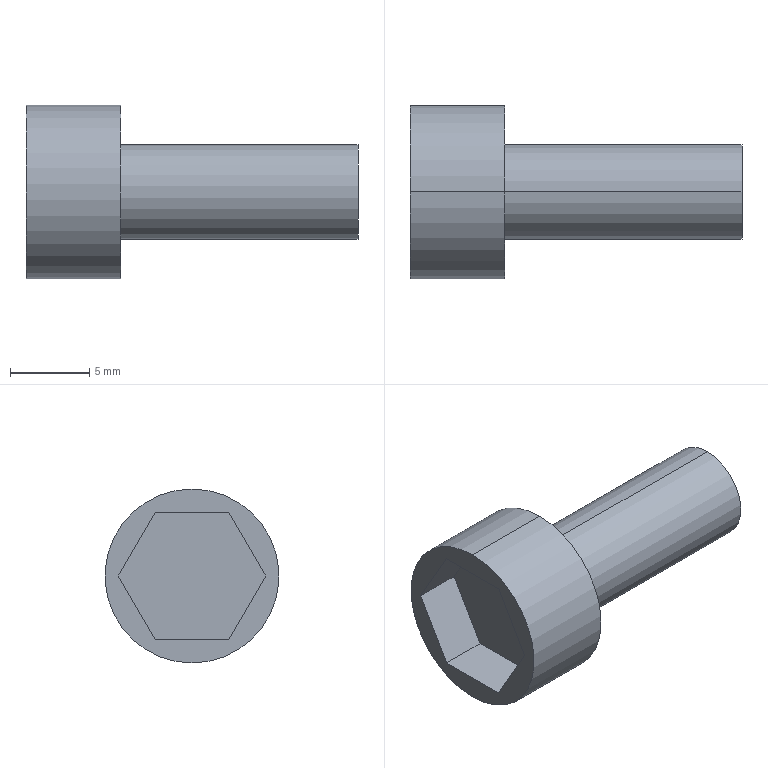Part | STEP file | M6 screw | 1 solid | 14 faces | box 21 x 11 x 11 mm | volume 825.269 mm3 | plane 10 | cylinder 4 | commonest cylinder face diameters 6 x2 11 x2
STEP:
#1=CARTESIAN_POINT('',(0.,0.,0.));
#2=DIRECTION('',(0.,0.,1.));
#3=DIRECTION('',(1.,0.,0.));
#4=AXIS2_PLACEMENT_3D('',#1,#2,#3);
#5=CARTESIAN_POINT('',(-7.171,-5.398,5.5));
#6=VERTEX_POINT('',#5);
#7=CARTESIAN_POINT('',(-7.171,-5.398,-5.5));
#8=VERTEX_POINT('',#7);
#9=CARTESIAN_POINT('',(-7.171,-5.398,0.));
#10=DIRECTION('',(-1.,0.,0.));
#11=DIRECTION('',(0.,0.,1.));
#12=AXIS2_PLACEMENT_3D('',#9,#10,#11);
#13=CIRCLE('',#12,5.5);
#14=CARTESIAN_POINT('',(-13.171,-5.398,0.));
#15=DIRECTION('',(-1.,0.,0.));
#16=DIRECTION('',(0.,0.,1.));
#17=AXIS2_PLACEMENT_3D('',#14,#15,#16);
#18=CYLINDRICAL_SURFACE('',#17,5.5);
#19=CARTESIAN_POINT('',(0.,-6.));
#20=DIRECTION('',(1.,0.));
#21=VECTOR('',#20,1.);
#22=LINE('',#19,#21);
#23=(GEOMETRIC_REPRESENTATION_CONTEXT(2)PARAMETRIC_REPRESENTATION_CONTEXT()REPRESENTATION_CONTEXT('',''));
#24=DEFINITIONAL_REPRESENTATION('',(#22),#23);
#25=PCURVE('',#18,#24);
#26=CARTESIAN_POINT('',(-7.171,0.102,0.));
#27=DIRECTION('',(-1.,0.,0.));
#28=DIRECTION('',(0.,0.,1.));
#29=AXIS2_PLACEMENT_3D('',#26,#27,#28);
#30=PLANE('',#29);
#31=CARTESIAN_POINT('',(0.,-5.5));
#32=DIRECTION('',(1.,0.));
#33=AXIS2_PLACEMENT_2D('',#31,#32);
#34=CIRCLE('',#33,5.5);
#35=(GEOMETRIC_REPRESENTATION_CONTEXT(2)PARAMETRIC_REPRESENTATION_CONTEXT()REPRESENTATION_CONTEXT('',''));
#36=DEFINITIONAL_REPRESENTATION('',(#34),#35);
#37=PCURVE('',#30,#36);
#38=SURFACE_CURVE('',#13,(#25,#37),.PCURVE_S1.);
#39=EDGE_CURVE('',#6,#8,#38,.T.);
#40=ORIENTED_EDGE('',*,*,#39,.T.);
#41=CARTESIAN_POINT('',(-13.171,-5.398,-5.5));
#42=VERTEX_POINT('',#41);
#43=CARTESIAN_POINT('',(-13.171,-5.398,-5.5));
#44=DIRECTION('',(-1.,0.,0.));
#45=VECTOR('',#44,1.);
#46=LINE('',#43,#45);
#47=CARTESIAN_POINT('',(3.142,0.));
#48=DIRECTION('',(0.,1.));
#49=VECTOR('',#48,1.);
#50=LINE('',#47,#49);
#51=(GEOMETRIC_REPRESENTATION_CONTEXT(2)PARAMETRIC_REPRESENTATION_CONTEXT()REPRESENTATION_CONTEXT('',''));
#52=DEFINITIONAL_REPRESENTATION('',(#50),#51);
#53=PCURVE('',#18,#52);
#54=CARTESIAN_POINT('',(-13.171,-5.398,0.));
#55=DIRECTION('',(-1.,0.,0.));
#56=DIRECTION('',(0.,0.,1.));
#57=AXIS2_PLACEMENT_3D('',#54,#55,#56);
#58=CYLINDRICAL_SURFACE('',#57,5.5);
#59=CARTESIAN_POINT('',(3.142,0.));
#60=DIRECTION('',(0.,1.));
#61=VECTOR('',#60,1.);
#62=LINE('',#59,#61);
#63=(GEOMETRIC_REPRESENTATION_CONTEXT(2)PARAMETRIC_REPRESENTATION_CONTEXT()REPRESENTATION_CONTEXT('',''));
#64=DEFINITIONAL_REPRESENTATION('',(#62),#63);
#65=PCURVE('',#58,#64);
#66=SURFACE_CURVE('',#46,(#53,#65),.PCURVE_S1.);
#67=EDGE_CURVE('',#8,#42,#66,.T.);
#68=ORIENTED_EDGE('',*,*,#67,.T.);
#69=CARTESIAN_POINT('',(-13.171,-5.398,5.5));
#70=VERTEX_POINT('',#69);
#71=CARTESIAN_POINT('',(-13.171,-5.398,0.));
#72=DIRECTION('',(-1.,0.,0.));
#73=DIRECTION('',(0.,0.,1.));
#74=AXIS2_PLACEMENT_3D('',#71,#72,#73);
#75=CIRCLE('',#74,5.5);
#76=CARTESIAN_POINT('',(0.,0.));
#77=DIRECTION('',(1.,0.));
#78=VECTOR('',#77,1.);
#79=LINE('',#76,#78);
#80=(GEOMETRIC_REPRESENTATION_CONTEXT(2)PARAMETRIC_REPRESENTATION_CONTEXT()REPRESENTATION_CONTEXT('',''));
#81=DEFINITIONAL_REPRESENTATION('',(#79),#80);
#82=PCURVE('',#18,#81);
#83=CARTESIAN_POINT('',(-13.171,0.102,0.));
#84=DIRECTION('',(1.,0.,0.));
#85=DIRECTION('',(0.,0.,-1.));
#86=AXIS2_PLACEMENT_3D('',#83,#84,#85);
#87=PLANE('',#86);
#88=CARTESIAN_POINT('',(-5.5,-5.5));
#89=CARTESIAN_POINT('',(-5.5,4.026));
#90=CARTESIAN_POINT('',(2.75,-0.7369));
#91=CARTESIAN_POINT('',(11.,-5.5));
#92=CARTESIAN_POINT('',(2.75,-10.263));
#93=CARTESIAN_POINT('',(-5.5,-15.026));
#94=CARTESIAN_POINT('',(-5.5,-5.5));
#95=(BOUNDED_CURVE()B_SPLINE_CURVE(2,(#88,#89,#90,#91,#92,#93,#94),.UNSPECIFIED.,.T.,.F.)B_SPLINE_CURVE_WITH_KNOTS((1,2,2,2,2,1),(-2.094,0.,2.094,4.189,6.283,8.378),.UNSPECIFIED.)CURVE()GEOMETRIC_REPRESENTATION_ITEM()RATIONAL_B_SPLINE_CURVE((1.,0.5,1.,0.5,1.,0.5,1.))REPRESENTATION_ITEM(''));
#96=(GEOMETRIC_REPRESENTATION_CONTEXT(2)PARAMETRIC_REPRESENTATION_CONTEXT()REPRESENTATION_CONTEXT('',''));
#97=DEFINITIONAL_REPRESENTATION('',(#95),#96);
#98=PCURVE('',#87,#97);
#99=SURFACE_CURVE('',#75,(#82,#98),.PCURVE_S1.);
#100=EDGE_CURVE('',#70,#42,#99,.T.);
#101=ORIENTED_EDGE('',*,*,#100,.F.);
#102=CARTESIAN_POINT('',(-13.171,-5.398,5.5));
#103=DIRECTION('',(-1.,0.,0.));
#104=VECTOR('',#103,1.);
#105=LINE('',#102,#104);
#106=CARTESIAN_POINT('',(0.,0.));
#107=DIRECTION('',(0.,1.));
#108=VECTOR('',#107,1.);
#109=LINE('',#106,#108);
#110=(GEOMETRIC_REPRESENTATION_CONTEXT(2)PARAMETRIC_REPRESENTATION_CONTEXT()REPRESENTATION_CONTEXT('',''));
#111=DEFINITIONAL_REPRESENTATION('',(#109),#110);
#112=PCURVE('',#18,#111);
#113=CARTESIAN_POINT('',(6.283,0.));
#114=DIRECTION('',(0.,1.));
#115=VECTOR('',#114,1.);
#116=LINE('',#113,#115);
#117=(GEOMETRIC_REPRESENTATION_CONTEXT(2)PARAMETRIC_REPRESENTATION_CONTEXT()REPRESENTATION_CONTEXT('',''));
#118=DEFINITIONAL_REPRESENTATION('',(#116),#117);
#119=PCURVE('',#58,#118);
#120=SURFACE_CURVE('',#105,(#112,#119),.PCURVE_S1.);
#121=EDGE_CURVE('',#6,#70,#120,.T.);
#122=ORIENTED_EDGE('',*,*,#121,.F.);
#123=EDGE_LOOP('',(#40,#68,#101,#122));
#124=FACE_BOUND('',#123,.T.);
#125=ADVANCED_FACE('',(#124),#18,.T.);
#126=CARTESIAN_POINT('',(7.829,-5.398,3.));
#127=VERTEX_POINT('',#126);
#128=CARTESIAN_POINT('',(7.829,-5.398,-3.));
#129=VERTEX_POINT('',#128);
#130=CARTESIAN_POINT('',(7.829,-5.398,0.));
#131=DIRECTION('',(-1.,0.,0.));
#132=DIRECTION('',(0.,0.,1.));
#133=AXIS2_PLACEMENT_3D('',#130,#131,#132);
#134=CIRCLE('',#133,3.);
#135=CARTESIAN_POINT('',(-13.171,-5.398,0.));
#136=DIRECTION('',(-1.,0.,0.));
#137=DIRECTION('',(0.,0.,1.));
#138=AXIS2_PLACEMENT_3D('',#135,#136,#137);
#139=CYLINDRICAL_SURFACE('',#138,3.);
#140=CARTESIAN_POINT('',(0.,-21.));
#141=DIRECTION('',(1.,0.));
#142=VECTOR('',#141,1.);
#143=LINE('',#140,#142);
#144=(GEOMETRIC_REPRESENTATION_CONTEXT(2)PARAMETRIC_REPRESENTATION_CONTEXT()REPRESENTATION_CONTEXT('',''));
#145=DEFINITIONAL_REPRESENTATION('',(#143),#144);
#146=PCURVE('',#139,#145);
#147=CARTESIAN_POINT('',(7.829,-5.398,0.));
#148=DIRECTION('',(-1.,0.,0.));
#149=DIRECTION('',(0.,0.,1.));
#150=AXIS2_PLACEMENT_3D('',#147,#148,#149);
#151=PLANE('',#150);
#152=CARTESIAN_POINT('',(0.,0.));
#153=DIRECTION('',(1.,0.));
#154=AXIS2_PLACEMENT_2D('',#152,#153);
#155=CIRCLE('',#154,3.);
#156=(GEOMETRIC_REPRESENTATION_CONTEXT(2)PARAMETRIC_REPRESENTATION_CONTEXT()REPRESENTATION_CONTEXT('',''));
#157=DEFINITIONAL_REPRESENTATION('',(#155),#156);
#158=PCURVE('',#151,#157);
#159=SURFACE_CURVE('',#134,(#146,#158),.PCURVE_S1.);
#160=EDGE_CURVE('',#127,#129,#159,.T.);
#161=ORIENTED_EDGE('',*,*,#160,.T.);
#162=CARTESIAN_POINT('',(-7.171,-5.398,-3.));
#163=VERTEX_POINT('',#162);
#164=CARTESIAN_POINT('',(-13.171,-5.398,-3.));
#165=DIRECTION('',(-1.,0.,0.));
#166=VECTOR('',#165,1.);
#167=LINE('',#164,#166);
#168=CARTESIAN_POINT('',(3.142,0.));
#169=DIRECTION('',(0.,1.));
#170=VECTOR('',#169,1.);
#171=LINE('',#168,#170);
#172=(GEOMETRIC_REPRESENTATION_CONTEXT(2)PARAMETRIC_REPRESENTATION_CONTEXT()REPRESENTATION_CONTEXT('',''));
#173=DEFINITIONAL_REPRESENTATION('',(#171),#172);
#174=PCURVE('',#139,#173);
#175=CARTESIAN_POINT('',(-13.171,-5.398,0.));
#176=DIRECTION('',(-1.,0.,0.));
#177=DIRECTION('',(0.,0.,1.));
#178=AXIS2_PLACEMENT_3D('',#175,#176,#177);
#179=CYLINDRICAL_SURFACE('',#178,3.);
#180=CARTESIAN_POINT('',(3.142,0.));
#181=DIRECTION('',(0.,1.));
#182=VECTOR('',#181,1.);
#183=LINE('',#180,#182);
#184=(GEOMETRIC_REPRESENTATION_CONTEXT(2)PARAMETRIC_REPRESENTATION_CONTEXT()REPRESENTATION_CONTEXT('',''));
#185=DEFINITIONAL_REPRESENTATION('',(#183),#184);
#186=PCURVE('',#179,#185);
#187=SURFACE_CURVE('',#167,(#174,#186),.PCURVE_S1.);
#188=EDGE_CURVE('',#129,#163,#187,.T.);
#189=ORIENTED_EDGE('',*,*,#188,.T.);
#190=CARTESIAN_POINT('',(-7.171,-5.398,3.));
#191=VERTEX_POINT('',#190);
#192=CARTESIAN_POINT('',(-7.171,-5.398,0.));
#193=DIRECTION('',(-1.,0.,0.));
#194=DIRECTION('',(0.,0.,1.));
#195=AXIS2_PLACEMENT_3D('',#192,#193,#194);
#196=CIRCLE('',#195,3.);
#197=CARTESIAN_POINT('',(0.,-6.));
#198=DIRECTION('',(1.,0.));
#199=VECTOR('',#198,1.);
#200=LINE('',#197,#199);
#201=(GEOMETRIC_REPRESENTATION_CONTEXT(2)PARAMETRIC_REPRESENTATION_CONTEXT()REPRESENTATION_CONTEXT('',''));
#202=DEFINITIONAL_REPRESENTATION('',(#200),#201);
#203=PCURVE('',#139,#202);
#204=CARTESIAN_POINT('',(0.,-5.5));
#205=DIRECTION('',(1.,0.));
#206=AXIS2_PLACEMENT_2D('',#204,#205);
#207=CIRCLE('',#206,3.);
#208=(GEOMETRIC_REPRESENTATION_CONTEXT(2)PARAMETRIC_REPRESENTATION_CONTEXT()REPRESENTATION_CONTEXT('',''));
#209=DEFINITIONAL_REPRESENTATION('',(#207),#208);
#210=PCURVE('',#30,#209);
#211=SURFACE_CURVE('',#196,(#203,#210),.PCURVE_S1.);
#212=EDGE_CURVE('',#191,#163,#211,.T.);
#213=ORIENTED_EDGE('',*,*,#212,.F.);
#214=CARTESIAN_POINT('',(-13.171,-5.398,3.));
#215=DIRECTION('',(-1.,0.,0.));
#216=VECTOR('',#215,1.);
#217=LINE('',#214,#216);
#218=CARTESIAN_POINT('',(0.,0.));
#219=DIRECTION('',(0.,1.));
#220=VECTOR('',#219,1.);
#221=LINE('',#218,#220);
#222=(GEOMETRIC_REPRESENTATION_CONTEXT(2)PARAMETRIC_REPRESENTATION_CONTEXT()REPRESENTATION_CONTEXT('',''));
#223=DEFINITIONAL_REPRESENTATION('',(#221),#222);
#224=PCURVE('',#139,#223);
#225=CARTESIAN_POINT('',(6.283,0.));
#226=DIRECTION('',(0.,1.));
#227=VECTOR('',#226,1.);
#228=LINE('',#225,#227);
#229=(GEOMETRIC_REPRESENTATION_CONTEXT(2)PARAMETRIC_REPRESENTATION_CONTEXT()REPRESENTATION_CONTEXT('',''));
#230=DEFINITIONAL_REPRESENTATION('',(#228),#229);
#231=PCURVE('',#179,#230);
#232=SURFACE_CURVE('',#217,(#224,#231),.PCURVE_S1.);
#233=EDGE_CURVE('',#127,#191,#232,.T.);
#234=ORIENTED_EDGE('',*,*,#233,.F.);
#235=EDGE_LOOP('',(#161,#189,#213,#234));
#236=FACE_BOUND('',#235,.T.);
#237=ADVANCED_FACE('',(#236),#139,.T.);
#238=CARTESIAN_POINT('',(-13.171,-10.055,0.));
#239=VERTEX_POINT('',#238);
#240=CARTESIAN_POINT('',(-13.171,-7.727,4.033));
#241=VERTEX_POINT('',#240);
#242=CARTESIAN_POINT('',(-13.171,-10.055,0.));
#243=DIRECTION('',(0.,0.5,0.866));
#244=VECTOR('',#243,1.);
#245=LINE('',#242,#244);
#246=CARTESIAN_POINT('',(0.,-10.157));
#247=DIRECTION('',(-0.866,0.5));
#248=VECTOR('',#247,1.);
#249=LINE('',#246,#248);
#250=(GEOMETRIC_REPRESENTATION_CONTEXT(2)PARAMETRIC_REPRESENTATION_CONTEXT()REPRESENTATION_CONTEXT('',''));
#251=DEFINITIONAL_REPRESENTATION('',(#249),#250);
#252=PCURVE('',#87,#251);
#253=CARTESIAN_POINT('',(-10.171,-10.055,0.));
#254=DIRECTION('',(0.,-0.866,0.5));
#255=DIRECTION('',(0.,-0.5,-0.866));
#256=AXIS2_PLACEMENT_3D('',#253,#254,#255);
#257=PLANE('',#256);
#258=CARTESIAN_POINT('',(0.,-3.));
#259=DIRECTION('',(-1.,0.));
#260=VECTOR('',#259,1.);
#261=LINE('',#258,#260);
#262=(GEOMETRIC_REPRESENTATION_CONTEXT(2)PARAMETRIC_REPRESENTATION_CONTEXT()REPRESENTATION_CONTEXT('',''));
#263=DEFINITIONAL_REPRESENTATION('',(#261),#262);
#264=PCURVE('',#257,#263);
#265=SURFACE_CURVE('',#245,(#252,#264),.PCURVE_S1.);
#266=EDGE_CURVE('',#239,#241,#265,.T.);
#267=ORIENTED_EDGE('',*,*,#266,.F.);
#268=CARTESIAN_POINT('',(-13.171,-7.727,-4.033));
#269=VERTEX_POINT('',#268);
#270=CARTESIAN_POINT('',(-13.171,-7.727,-4.033));
#271=DIRECTION('',(0.,-0.5,0.866));
#272=VECTOR('',#271,1.);
#273=LINE('',#270,#272);
#274=CARTESIAN_POINT('',(4.033,-7.829));
#275=DIRECTION('',(-0.866,-0.5));
#276=VECTOR('',#275,1.);
#277=LINE('',#274,#276);
#278=(GEOMETRIC_REPRESENTATION_CONTEXT(2)PARAMETRIC_REPRESENTATION_CONTEXT()REPRESENTATION_CONTEXT('',''));
#279=DEFINITIONAL_REPRESENTATION('',(#277),#278);
#280=PCURVE('',#87,#279);
#281=CARTESIAN_POINT('',(-10.171,-7.727,-4.033));
#282=DIRECTION('',(0.,-0.866,-0.5));
#283=DIRECTION('',(0.,0.5,-0.866));
#284=AXIS2_PLACEMENT_3D('',#281,#282,#283);
#285=PLANE('',#284);
#286=CARTESIAN_POINT('',(0.,-3.));
#287=DIRECTION('',(-1.,0.));
#288=VECTOR('',#287,1.);
#289=LINE('',#286,#288);
#290=(GEOMETRIC_REPRESENTATION_CONTEXT(2)PARAMETRIC_REPRESENTATION_CONTEXT()REPRESENTATION_CONTEXT('',''));
#291=DEFINITIONAL_REPRESENTATION('',(#289),#290);
#292=PCURVE('',#285,#291);
#293=SURFACE_CURVE('',#273,(#280,#292),.PCURVE_S1.);
#294=EDGE_CURVE('',#269,#239,#293,.T.);
#295=ORIENTED_EDGE('',*,*,#294,.F.);
#296=CARTESIAN_POINT('',(-13.171,-3.069,-4.033));
#297=VERTEX_POINT('',#296);
#298=CARTESIAN_POINT('',(-13.171,-3.069,-4.033));
#299=DIRECTION('',(0.,-1.,0.));
#300=VECTOR('',#299,1.);
#301=LINE('',#298,#300);
#302=CARTESIAN_POINT('',(4.033,-3.171));
#303=DIRECTION('',(0.,-1.));
#304=VECTOR('',#303,1.);
#305=LINE('',#302,#304);
#306=(GEOMETRIC_REPRESENTATION_CONTEXT(2)PARAMETRIC_REPRESENTATION_CONTEXT()REPRESENTATION_CONTEXT('',''));
#307=DEFINITIONAL_REPRESENTATION('',(#305),#306);
#308=PCURVE('',#87,#307);
#309=CARTESIAN_POINT('',(-10.171,-3.069,-4.033));
#310=DIRECTION('',(0.,0.,-1.));
#311=DIRECTION('',(0.,1.,0.));
#312=AXIS2_PLACEMENT_3D('',#309,#310,#311);
#313=PLANE('',#312);
#314=CARTESIAN_POINT('',(0.,-3.));
#315=DIRECTION('',(-1.,0.));
#316=VECTOR('',#315,1.);
#317=LINE('',#314,#316);
#318=(GEOMETRIC_REPRESENTATION_CONTEXT(2)PARAMETRIC_REPRESENTATION_CONTEXT()REPRESENTATION_CONTEXT('',''));
#319=DEFINITIONAL_REPRESENTATION('',(#317),#318);
#320=PCURVE('',#313,#319);
#321=SURFACE_CURVE('',#301,(#308,#320),.PCURVE_S1.);
#322=EDGE_CURVE('',#297,#269,#321,.T.);
#323=ORIENTED_EDGE('',*,*,#322,.F.);
#324=CARTESIAN_POINT('',(-13.171,-0.7409,0.));
#325=VERTEX_POINT('',#324);
#326=CARTESIAN_POINT('',(-13.171,-0.7409,0.));
#327=DIRECTION('',(0.,-0.5,-0.866));
#328=VECTOR('',#327,1.);
#329=LINE('',#326,#328);
#330=CARTESIAN_POINT('',(0.,-0.8429));
#331=DIRECTION('',(0.866,-0.5));
#332=VECTOR('',#331,1.);
#333=LINE('',#330,#332);
#334=(GEOMETRIC_REPRESENTATION_CONTEXT(2)PARAMETRIC_REPRESENTATION_CONTEXT()REPRESENTATION_CONTEXT('',''));
#335=DEFINITIONAL_REPRESENTATION('',(#333),#334);
#336=PCURVE('',#87,#335);
#337=CARTESIAN_POINT('',(-10.171,-0.7409,0.));
#338=DIRECTION('',(0.,0.866,-0.5));
#339=DIRECTION('',(0.,0.5,0.866));
#340=AXIS2_PLACEMENT_3D('',#337,#338,#339);
#341=PLANE('',#340);
#342=CARTESIAN_POINT('',(0.,-3.));
#343=DIRECTION('',(-1.,0.));
#344=VECTOR('',#343,1.);
#345=LINE('',#342,#344);
#346=(GEOMETRIC_REPRESENTATION_CONTEXT(2)PARAMETRIC_REPRESENTATION_CONTEXT()REPRESENTATION_CONTEXT('',''));
#347=DEFINITIONAL_REPRESENTATION('',(#345),#346);
#348=PCURVE('',#341,#347);
#349=SURFACE_CURVE('',#329,(#336,#348),.PCURVE_S1.);
#350=EDGE_CURVE('',#325,#297,#349,.T.);
#351=ORIENTED_EDGE('',*,*,#350,.F.);
#352=CARTESIAN_POINT('',(-13.171,-3.069,4.033));
#353=VERTEX_POINT('',#352);
#354=CARTESIAN_POINT('',(-13.171,-3.069,4.033));
#355=DIRECTION('',(0.,0.5,-0.866));
#356=VECTOR('',#355,1.);
#357=LINE('',#354,#356);
#358=CARTESIAN_POINT('',(-4.033,-3.171));
#359=DIRECTION('',(0.866,0.5));
#360=VECTOR('',#359,1.);
#361=LINE('',#358,#360);
#362=(GEOMETRIC_REPRESENTATION_CONTEXT(2)PARAMETRIC_REPRESENTATION_CONTEXT()REPRESENTATION_CONTEXT('',''));
#363=DEFINITIONAL_REPRESENTATION('',(#361),#362);
#364=PCURVE('',#87,#363);
#365=CARTESIAN_POINT('',(-10.171,-3.069,4.033));
#366=DIRECTION('',(0.,0.866,0.5));
#367=DIRECTION('',(0.,-0.5,0.866));
#368=AXIS2_PLACEMENT_3D('',#365,#366,#367);
#369=PLANE('',#368);
#370=CARTESIAN_POINT('',(0.,-3.));
#371=DIRECTION('',(-1.,0.));
#372=VECTOR('',#371,1.);
#373=LINE('',#370,#372);
#374=(GEOMETRIC_REPRESENTATION_CONTEXT(2)PARAMETRIC_REPRESENTATION_CONTEXT()REPRESENTATION_CONTEXT('',''));
#375=DEFINITIONAL_REPRESENTATION('',(#373),#374);
#376=PCURVE('',#369,#375);
#377=SURFACE_CURVE('',#357,(#364,#376),.PCURVE_S1.);
#378=EDGE_CURVE('',#353,#325,#377,.T.);
#379=ORIENTED_EDGE('',*,*,#378,.F.);
#380=CARTESIAN_POINT('',(-13.171,-7.727,4.033));
#381=DIRECTION('',(0.,1.,0.));
#382=VECTOR('',#381,1.);
#383=LINE('',#380,#382);
#384=CARTESIAN_POINT('',(-4.033,-7.829));
#385=DIRECTION('',(0.,1.));
#386=VECTOR('',#385,1.);
#387=LINE('',#384,#386);
#388=(GEOMETRIC_REPRESENTATION_CONTEXT(2)PARAMETRIC_REPRESENTATION_CONTEXT()REPRESENTATION_CONTEXT('',''));
#389=DEFINITIONAL_REPRESENTATION('',(#387),#388);
#390=PCURVE('',#87,#389);
#391=CARTESIAN_POINT('',(-10.171,-7.727,4.033));
#392=DIRECTION('',(0.,0.,1.));
#393=DIRECTION('',(0.,-1.,0.));
#394=AXIS2_PLACEMENT_3D('',#391,#392,#393);
#395=PLANE('',#394);
#396=CARTESIAN_POINT('',(0.,-3.));
#397=DIRECTION('',(-1.,0.));
#398=VECTOR('',#397,1.);
#399=LINE('',#396,#398);
#400=(GEOMETRIC_REPRESENTATION_CONTEXT(2)PARAMETRIC_REPRESENTATION_CONTEXT()REPRESENTATION_CONTEXT('',''));
#401=DEFINITIONAL_REPRESENTATION('',(#399),#400);
#402=PCURVE('',#395,#401);
#403=SURFACE_CURVE('',#383,(#390,#402),.PCURVE_S1.);
#404=EDGE_CURVE('',#241,#353,#403,.T.);
#405=ORIENTED_EDGE('',*,*,#404,.F.);
#406=EDGE_LOOP('',(#267,#295,#323,#351,#379,#405));
#407=FACE_BOUND('',#406,.T.);
#408=ORIENTED_EDGE('',*,*,#100,.T.);
#409=CARTESIAN_POINT('',(-13.171,-5.398,0.));
#410=DIRECTION('',(-1.,0.,0.));
#411=DIRECTION('',(0.,0.,1.));
#412=AXIS2_PLACEMENT_3D('',#409,#410,#411);
#413=CIRCLE('',#412,5.5);
#414=CARTESIAN_POINT('',(-5.5,-5.5));
#415=CARTESIAN_POINT('',(-5.5,4.026));
#416=CARTESIAN_POINT('',(2.75,-0.7369));
#417=CARTESIAN_POINT('',(11.,-5.5));
#418=CARTESIAN_POINT('',(2.75,-10.263));
#419=CARTESIAN_POINT('',(-5.5,-15.026));
#420=CARTESIAN_POINT('',(-5.5,-5.5));
#421=(BOUNDED_CURVE()B_SPLINE_CURVE(2,(#414,#415,#416,#417,#418,#419,#420),.UNSPECIFIED.,.T.,.F.)B_SPLINE_CURVE_WITH_KNOTS((1,2,2,2,2,1),(-2.094,0.,2.094,4.189,6.283,8.378),.UNSPECIFIED.)CURVE()GEOMETRIC_REPRESENTATION_ITEM()RATIONAL_B_SPLINE_CURVE((1.,0.5,1.,0.5,1.,0.5,1.))REPRESENTATION_ITEM(''));
#422=(GEOMETRIC_REPRESENTATION_CONTEXT(2)PARAMETRIC_REPRESENTATION_CONTEXT()REPRESENTATION_CONTEXT('',''));
#423=DEFINITIONAL_REPRESENTATION('',(#421),#422);
#424=PCURVE('',#87,#423);
#425=CARTESIAN_POINT('',(0.,0.));
#426=DIRECTION('',(1.,0.));
#427=VECTOR('',#426,1.);
#428=LINE('',#425,#427);
#429=(GEOMETRIC_REPRESENTATION_CONTEXT(2)PARAMETRIC_REPRESENTATION_CONTEXT()REPRESENTATION_CONTEXT('',''));
#430=DEFINITIONAL_REPRESENTATION('',(#428),#429);
#431=PCURVE('',#58,#430);
#432=SURFACE_CURVE('',#413,(#424,#431),.PCURVE_S1.);
#433=EDGE_CURVE('',#42,#70,#432,.T.);
#434=ORIENTED_EDGE('',*,*,#433,.T.);
#435=EDGE_LOOP('',(#408,#434));
#436=FACE_BOUND('',#435,.T.);
#437=ADVANCED_FACE('',(#407,#436),#87,.F.);
#438=ORIENTED_EDGE('',*,*,#160,.F.);
#439=CARTESIAN_POINT('',(7.829,-5.398,0.));
#440=DIRECTION('',(-1.,0.,0.));
#441=DIRECTION('',(0.,0.,1.));
#442=AXIS2_PLACEMENT_3D('',#439,#440,#441);
#443=CIRCLE('',#442,3.);
#444=CARTESIAN_POINT('',(0.,0.));
#445=DIRECTION('',(1.,0.));
#446=AXIS2_PLACEMENT_2D('',#444,#445);
#447=CIRCLE('',#446,3.);
#448=(GEOMETRIC_REPRESENTATION_CONTEXT(2)PARAMETRIC_REPRESENTATION_CONTEXT()REPRESENTATION_CONTEXT('',''));
#449=DEFINITIONAL_REPRESENTATION('',(#447),#448);
#450=PCURVE('',#151,#449);
#451=CARTESIAN_POINT('',(0.,-21.));
#452=DIRECTION('',(1.,0.));
#453=VECTOR('',#452,1.);
#454=LINE('',#451,#453);
#455=(GEOMETRIC_REPRESENTATION_CONTEXT(2)PARAMETRIC_REPRESENTATION_CONTEXT()REPRESENTATION_CONTEXT('',''));
#456=DEFINITIONAL_REPRESENTATION('',(#454),#455);
#457=PCURVE('',#179,#456);
#458=SURFACE_CURVE('',#443,(#450,#457),.PCURVE_S1.);
#459=EDGE_CURVE('',#129,#127,#458,.T.);
#460=ORIENTED_EDGE('',*,*,#459,.F.);
#461=EDGE_LOOP('',(#438,#460));
#462=FACE_BOUND('',#461,.T.);
#463=ADVANCED_FACE('',(#462),#151,.F.);
#464=ORIENTED_EDGE('',*,*,#188,.F.);
#465=ORIENTED_EDGE('',*,*,#459,.T.);
#466=ORIENTED_EDGE('',*,*,#233,.T.);
#467=CARTESIAN_POINT('',(-7.171,-5.398,0.));
#468=DIRECTION('',(-1.,0.,0.));
#469=DIRECTION('',(0.,0.,1.));
#470=AXIS2_PLACEMENT_3D('',#467,#468,#469);
#471=CIRCLE('',#470,3.);
#472=CARTESIAN_POINT('',(0.,-6.));
#473=DIRECTION('',(1.,0.));
#474=VECTOR('',#473,1.);
#475=LINE('',#472,#474);
#476=(GEOMETRIC_REPRESENTATION_CONTEXT(2)PARAMETRIC_REPRESENTATION_CONTEXT()REPRESENTATION_CONTEXT('',''));
#477=DEFINITIONAL_REPRESENTATION('',(#475),#476);
#478=PCURVE('',#179,#477);
#479=CARTESIAN_POINT('',(0.,-5.5));
#480=DIRECTION('',(1.,0.));
#481=AXIS2_PLACEMENT_2D('',#479,#480);
#482=CIRCLE('',#481,3.);
#483=(GEOMETRIC_REPRESENTATION_CONTEXT(2)PARAMETRIC_REPRESENTATION_CONTEXT()REPRESENTATION_CONTEXT('',''));
#484=DEFINITIONAL_REPRESENTATION('',(#482),#483);
#485=PCURVE('',#30,#484);
#486=SURFACE_CURVE('',#471,(#478,#485),.PCURVE_S1.);
#487=EDGE_CURVE('',#163,#191,#486,.T.);
#488=ORIENTED_EDGE('',*,*,#487,.F.);
#489=EDGE_LOOP('',(#464,#465,#466,#488));
#490=FACE_BOUND('',#489,.T.);
#491=ADVANCED_FACE('',(#490),#179,.T.);
#492=ORIENTED_EDGE('',*,*,#39,.F.);
#493=CARTESIAN_POINT('',(-7.171,-5.398,0.));
#494=DIRECTION('',(-1.,0.,0.));
#495=DIRECTION('',(0.,0.,1.));
#496=AXIS2_PLACEMENT_3D('',#493,#494,#495);
#497=CIRCLE('',#496,5.5);
#498=CARTESIAN_POINT('',(0.,-5.5));
#499=DIRECTION('',(1.,0.));
#500=AXIS2_PLACEMENT_2D('',#498,#499);
#501=CIRCLE('',#500,5.5);
#502=(GEOMETRIC_REPRESENTATION_CONTEXT(2)PARAMETRIC_REPRESENTATION_CONTEXT()REPRESENTATION_CONTEXT('',''));
#503=DEFINITIONAL_REPRESENTATION('',(#501),#502);
#504=PCURVE('',#30,#503);
#505=CARTESIAN_POINT('',(0.,-6.));
#506=DIRECTION('',(1.,0.));
#507=VECTOR('',#506,1.);
#508=LINE('',#505,#507);
#509=(GEOMETRIC_REPRESENTATION_CONTEXT(2)PARAMETRIC_REPRESENTATION_CONTEXT()REPRESENTATION_CONTEXT('',''));
#510=DEFINITIONAL_REPRESENTATION('',(#508),#509);
#511=PCURVE('',#58,#510);
#512=SURFACE_CURVE('',#497,(#504,#511),.PCURVE_S1.);
#513=EDGE_CURVE('',#8,#6,#512,.T.);
#514=ORIENTED_EDGE('',*,*,#513,.F.);
#515=EDGE_LOOP('',(#492,#514));
#516=FACE_BOUND('',#515,.T.);
#517=ORIENTED_EDGE('',*,*,#212,.T.);
#518=ORIENTED_EDGE('',*,*,#487,.T.);
#519=EDGE_LOOP('',(#517,#518));
#520=FACE_BOUND('',#519,.T.);
#521=ADVANCED_FACE('',(#516,#520),#30,.F.);
#522=ORIENTED_EDGE('',*,*,#67,.F.);
#523=ORIENTED_EDGE('',*,*,#513,.T.);
#524=ORIENTED_EDGE('',*,*,#121,.T.);
#525=ORIENTED_EDGE('',*,*,#433,.F.);
#526=EDGE_LOOP('',(#522,#523,#524,#525));
#527=FACE_BOUND('',#526,.T.);
#528=ADVANCED_FACE('',(#527),#58,.T.);
#529=ORIENTED_EDGE('',*,*,#294,.T.);
#530=CARTESIAN_POINT('',(-10.171,-10.055,0.));
#531=VERTEX_POINT('',#530);
#532=CARTESIAN_POINT('',(-10.171,-10.055,0.));
#533=DIRECTION('',(-1.,0.,0.));
#534=VECTOR('',#533,1.);
#535=LINE('',#532,#534);
#536=CARTESIAN_POINT('',(-4.657,0.));
#537=DIRECTION('',(0.,-1.));
#538=VECTOR('',#537,1.);
#539=LINE('',#536,#538);
#540=(GEOMETRIC_REPRESENTATION_CONTEXT(2)PARAMETRIC_REPRESENTATION_CONTEXT()REPRESENTATION_CONTEXT('',''));
#541=DEFINITIONAL_REPRESENTATION('',(#539),#540);
#542=PCURVE('',#285,#541);
#543=CARTESIAN_POINT('',(0.,0.));
#544=DIRECTION('',(0.,-1.));
#545=VECTOR('',#544,1.);
#546=LINE('',#543,#545);
#547=(GEOMETRIC_REPRESENTATION_CONTEXT(2)PARAMETRIC_REPRESENTATION_CONTEXT()REPRESENTATION_CONTEXT('',''));
#548=DEFINITIONAL_REPRESENTATION('',(#546),#547);
#549=PCURVE('',#257,#548);
#550=SURFACE_CURVE('',#535,(#542,#549),.PCURVE_S1.);
#551=EDGE_CURVE('',#531,#239,#550,.T.);
#552=ORIENTED_EDGE('',*,*,#551,.F.);
#553=CARTESIAN_POINT('',(-10.171,-7.727,-4.033));
#554=VERTEX_POINT('',#553);
#555=CARTESIAN_POINT('',(-10.171,-7.727,-4.033));
#556=DIRECTION('',(0.,-0.5,0.866));
#557=VECTOR('',#556,1.);
#558=LINE('',#555,#557);
#559=CARTESIAN_POINT('',(0.,0.));
#560=DIRECTION('',(-1.,0.));
#561=VECTOR('',#560,1.);
#562=LINE('',#559,#561);
#563=(GEOMETRIC_REPRESENTATION_CONTEXT(2)PARAMETRIC_REPRESENTATION_CONTEXT()REPRESENTATION_CONTEXT('',''));
#564=DEFINITIONAL_REPRESENTATION('',(#562),#563);
#565=PCURVE('',#285,#564);
#566=CARTESIAN_POINT('',(-10.171,-12.384,4.033));
#567=DIRECTION('',(-1.,0.,0.));
#568=DIRECTION('',(0.,0.,1.));
#569=AXIS2_PLACEMENT_3D('',#566,#567,#568);
#570=PLANE('',#569);
#571=CARTESIAN_POINT('',(-8.066,4.657));
#572=DIRECTION('',(0.866,-0.5));
#573=VECTOR('',#572,1.);
#574=LINE('',#571,#573);
#575=(GEOMETRIC_REPRESENTATION_CONTEXT(2)PARAMETRIC_REPRESENTATION_CONTEXT()REPRESENTATION_CONTEXT('',''));
#576=DEFINITIONAL_REPRESENTATION('',(#574),#575);
#577=PCURVE('',#570,#576);
#578=SURFACE_CURVE('',#558,(#565,#577),.PCURVE_S1.);
#579=EDGE_CURVE('',#554,#531,#578,.T.);
#580=ORIENTED_EDGE('',*,*,#579,.F.);
#581=CARTESIAN_POINT('',(-10.171,-7.727,-4.033));
#582=DIRECTION('',(-1.,0.,0.));
#583=VECTOR('',#582,1.);
#584=LINE('',#581,#583);
#585=CARTESIAN_POINT('',(0.,0.));
#586=DIRECTION('',(0.,-1.));
#587=VECTOR('',#586,1.);
#588=LINE('',#585,#587);
#589=(GEOMETRIC_REPRESENTATION_CONTEXT(2)PARAMETRIC_REPRESENTATION_CONTEXT()REPRESENTATION_CONTEXT('',''));
#590=DEFINITIONAL_REPRESENTATION('',(#588),#589);
#591=PCURVE('',#285,#590);
#592=CARTESIAN_POINT('',(-4.657,0.));
#593=DIRECTION('',(0.,-1.));
#594=VECTOR('',#593,1.);
#595=LINE('',#592,#594);
#596=(GEOMETRIC_REPRESENTATION_CONTEXT(2)PARAMETRIC_REPRESENTATION_CONTEXT()REPRESENTATION_CONTEXT('',''));
#597=DEFINITIONAL_REPRESENTATION('',(#595),#596);
#598=PCURVE('',#313,#597);
#599=SURFACE_CURVE('',#584,(#591,#598),.PCURVE_S1.);
#600=EDGE_CURVE('',#554,#269,#599,.T.);
#601=ORIENTED_EDGE('',*,*,#600,.T.);
#602=EDGE_LOOP('',(#529,#552,#580,#601));
#603=FACE_BOUND('',#602,.T.);
#604=ADVANCED_FACE('',(#603),#285,.F.);
#605=ORIENTED_EDGE('',*,*,#322,.T.);
#606=ORIENTED_EDGE('',*,*,#600,.F.);
#607=CARTESIAN_POINT('',(-10.171,-3.069,-4.033));
#608=VERTEX_POINT('',#607);
#609=CARTESIAN_POINT('',(-10.171,-3.069,-4.033));
#610=DIRECTION('',(0.,-1.,0.));
#611=VECTOR('',#610,1.);
#612=LINE('',#609,#611);
#613=CARTESIAN_POINT('',(0.,0.));
#614=DIRECTION('',(-1.,0.));
#615=VECTOR('',#614,1.);
#616=LINE('',#613,#615);
#617=(GEOMETRIC_REPRESENTATION_CONTEXT(2)PARAMETRIC_REPRESENTATION_CONTEXT()REPRESENTATION_CONTEXT('',''));
#618=DEFINITIONAL_REPRESENTATION('',(#616),#617);
#619=PCURVE('',#313,#618);
#620=CARTESIAN_POINT('',(-8.066,9.314));
#621=DIRECTION('',(0.,-1.));
#622=VECTOR('',#621,1.);
#623=LINE('',#620,#622);
#624=(GEOMETRIC_REPRESENTATION_CONTEXT(2)PARAMETRIC_REPRESENTATION_CONTEXT()REPRESENTATION_CONTEXT('',''));
#625=DEFINITIONAL_REPRESENTATION('',(#623),#624);
#626=PCURVE('',#570,#625);
#627=SURFACE_CURVE('',#612,(#619,#626),.PCURVE_S1.);
#628=EDGE_CURVE('',#608,#554,#627,.T.);
#629=ORIENTED_EDGE('',*,*,#628,.F.);
#630=CARTESIAN_POINT('',(-10.171,-3.069,-4.033));
#631=DIRECTION('',(-1.,0.,0.));
#632=VECTOR('',#631,1.);
#633=LINE('',#630,#632);
#634=CARTESIAN_POINT('',(0.,0.));
#635=DIRECTION('',(0.,-1.));
#636=VECTOR('',#635,1.);
#637=LINE('',#634,#636);
#638=(GEOMETRIC_REPRESENTATION_CONTEXT(2)PARAMETRIC_REPRESENTATION_CONTEXT()REPRESENTATION_CONTEXT('',''));
#639=DEFINITIONAL_REPRESENTATION('',(#637),#638);
#640=PCURVE('',#313,#639);
#641=CARTESIAN_POINT('',(-4.657,0.));
#642=DIRECTION('',(0.,-1.));
#643=VECTOR('',#642,1.);
#644=LINE('',#641,#643);
#645=(GEOMETRIC_REPRESENTATION_CONTEXT(2)PARAMETRIC_REPRESENTATION_CONTEXT()REPRESENTATION_CONTEXT('',''));
#646=DEFINITIONAL_REPRESENTATION('',(#644),#645);
#647=PCURVE('',#341,#646);
#648=SURFACE_CURVE('',#633,(#640,#647),.PCURVE_S1.);
#649=EDGE_CURVE('',#608,#297,#648,.T.);
#650=ORIENTED_EDGE('',*,*,#649,.T.);
#651=EDGE_LOOP('',(#605,#606,#629,#650));
#652=FACE_BOUND('',#651,.T.);
#653=ADVANCED_FACE('',(#652),#313,.F.);
#654=ORIENTED_EDGE('',*,*,#350,.T.);
#655=ORIENTED_EDGE('',*,*,#649,.F.);
#656=CARTESIAN_POINT('',(-10.171,-0.7409,0.));
#657=VERTEX_POINT('',#656);
#658=CARTESIAN_POINT('',(-10.171,-0.7409,0.));
#659=DIRECTION('',(0.,-0.5,-0.866));
#660=VECTOR('',#659,1.);
#661=LINE('',#658,#660);
#662=CARTESIAN_POINT('',(0.,0.));
#663=DIRECTION('',(-1.,0.));
#664=VECTOR('',#663,1.);
#665=LINE('',#662,#664);
#666=(GEOMETRIC_REPRESENTATION_CONTEXT(2)PARAMETRIC_REPRESENTATION_CONTEXT()REPRESENTATION_CONTEXT('',''));
#667=DEFINITIONAL_REPRESENTATION('',(#665),#666);
#668=PCURVE('',#341,#667);
#669=CARTESIAN_POINT('',(-4.033,11.643));
#670=DIRECTION('',(-0.866,-0.5));
#671=VECTOR('',#670,1.);
#672=LINE('',#669,#671);
#673=(GEOMETRIC_REPRESENTATION_CONTEXT(2)PARAMETRIC_REPRESENTATION_CONTEXT()REPRESENTATION_CONTEXT('',''));
#674=DEFINITIONAL_REPRESENTATION('',(#672),#673);
#675=PCURVE('',#570,#674);
#676=SURFACE_CURVE('',#661,(#668,#675),.PCURVE_S1.);
#677=EDGE_CURVE('',#657,#608,#676,.T.);
#678=ORIENTED_EDGE('',*,*,#677,.F.);
#679=CARTESIAN_POINT('',(-10.171,-0.7409,0.));
#680=DIRECTION('',(-1.,0.,0.));
#681=VECTOR('',#680,1.);
#682=LINE('',#679,#681);
#683=CARTESIAN_POINT('',(0.,0.));
#684=DIRECTION('',(0.,-1.));
#685=VECTOR('',#684,1.);
#686=LINE('',#683,#685);
#687=(GEOMETRIC_REPRESENTATION_CONTEXT(2)PARAMETRIC_REPRESENTATION_CONTEXT()REPRESENTATION_CONTEXT('',''));
#688=DEFINITIONAL_REPRESENTATION('',(#686),#687);
#689=PCURVE('',#341,#688);
#690=CARTESIAN_POINT('',(-4.657,0.));
#691=DIRECTION('',(0.,-1.));
#692=VECTOR('',#691,1.);
#693=LINE('',#690,#692);
#694=(GEOMETRIC_REPRESENTATION_CONTEXT(2)PARAMETRIC_REPRESENTATION_CONTEXT()REPRESENTATION_CONTEXT('',''));
#695=DEFINITIONAL_REPRESENTATION('',(#693),#694);
#696=PCURVE('',#369,#695);
#697=SURFACE_CURVE('',#682,(#689,#696),.PCURVE_S1.);
#698=EDGE_CURVE('',#657,#325,#697,.T.);
#699=ORIENTED_EDGE('',*,*,#698,.T.);
#700=EDGE_LOOP('',(#654,#655,#678,#699));
#701=FACE_BOUND('',#700,.T.);
#702=ADVANCED_FACE('',(#701),#341,.F.);
#703=ORIENTED_EDGE('',*,*,#378,.T.);
#704=ORIENTED_EDGE('',*,*,#698,.F.);
#705=CARTESIAN_POINT('',(-10.171,-3.069,4.033));
#706=VERTEX_POINT('',#705);
#707=CARTESIAN_POINT('',(-10.171,-3.069,4.033));
#708=DIRECTION('',(0.,0.5,-0.866));
#709=VECTOR('',#708,1.);
#710=LINE('',#707,#709);
#711=CARTESIAN_POINT('',(0.,0.));
#712=DIRECTION('',(-1.,0.));
#713=VECTOR('',#712,1.);
#714=LINE('',#711,#713);
#715=(GEOMETRIC_REPRESENTATION_CONTEXT(2)PARAMETRIC_REPRESENTATION_CONTEXT()REPRESENTATION_CONTEXT('',''));
#716=DEFINITIONAL_REPRESENTATION('',(#714),#715);
#717=PCURVE('',#369,#716);
#718=CARTESIAN_POINT('',(0.,9.314));
#719=DIRECTION('',(-0.866,0.5));
#720=VECTOR('',#719,1.);
#721=LINE('',#718,#720);
#722=(GEOMETRIC_REPRESENTATION_CONTEXT(2)PARAMETRIC_REPRESENTATION_CONTEXT()REPRESENTATION_CONTEXT('',''));
#723=DEFINITIONAL_REPRESENTATION('',(#721),#722);
#724=PCURVE('',#570,#723);
#725=SURFACE_CURVE('',#710,(#717,#724),.PCURVE_S1.);
#726=EDGE_CURVE('',#706,#657,#725,.T.);
#727=ORIENTED_EDGE('',*,*,#726,.F.);
#728=CARTESIAN_POINT('',(-10.171,-3.069,4.033));
#729=DIRECTION('',(-1.,0.,0.));
#730=VECTOR('',#729,1.);
#731=LINE('',#728,#730);
#732=CARTESIAN_POINT('',(0.,0.));
#733=DIRECTION('',(0.,-1.));
#734=VECTOR('',#733,1.);
#735=LINE('',#732,#734);
#736=(GEOMETRIC_REPRESENTATION_CONTEXT(2)PARAMETRIC_REPRESENTATION_CONTEXT()REPRESENTATION_CONTEXT('',''));
#737=DEFINITIONAL_REPRESENTATION('',(#735),#736);
#738=PCURVE('',#369,#737);
#739=CARTESIAN_POINT('',(-4.657,0.));
#740=DIRECTION('',(0.,-1.));
#741=VECTOR('',#740,1.);
#742=LINE('',#739,#741);
#743=(GEOMETRIC_REPRESENTATION_CONTEXT(2)PARAMETRIC_REPRESENTATION_CONTEXT()REPRESENTATION_CONTEXT('',''));
#744=DEFINITIONAL_REPRESENTATION('',(#742),#743);
#745=PCURVE('',#395,#744);
#746=SURFACE_CURVE('',#731,(#738,#745),.PCURVE_S1.);
#747=EDGE_CURVE('',#706,#353,#746,.T.);
#748=ORIENTED_EDGE('',*,*,#747,.T.);
#749=EDGE_LOOP('',(#703,#704,#727,#748));
#750=FACE_BOUND('',#749,.T.);
#751=ADVANCED_FACE('',(#750),#369,.F.);
#752=ORIENTED_EDGE('',*,*,#404,.T.);
#753=ORIENTED_EDGE('',*,*,#747,.F.);
#754=CARTESIAN_POINT('',(-10.171,-7.727,4.033));
#755=VERTEX_POINT('',#754);
#756=CARTESIAN_POINT('',(-10.171,-7.727,4.033));
#757=DIRECTION('',(0.,1.,0.));
#758=VECTOR('',#757,1.);
#759=LINE('',#756,#758);
#760=CARTESIAN_POINT('',(0.,0.));
#761=DIRECTION('',(-1.,0.));
#762=VECTOR('',#761,1.);
#763=LINE('',#760,#762);
#764=(GEOMETRIC_REPRESENTATION_CONTEXT(2)PARAMETRIC_REPRESENTATION_CONTEXT()REPRESENTATION_CONTEXT('',''));
#765=DEFINITIONAL_REPRESENTATION('',(#763),#764);
#766=PCURVE('',#395,#765);
#767=CARTESIAN_POINT('',(0.,4.657));
#768=DIRECTION('',(0.,1.));
#769=VECTOR('',#768,1.);
#770=LINE('',#767,#769);
#771=(GEOMETRIC_REPRESENTATION_CONTEXT(2)PARAMETRIC_REPRESENTATION_CONTEXT()REPRESENTATION_CONTEXT('',''));
#772=DEFINITIONAL_REPRESENTATION('',(#770),#771);
#773=PCURVE('',#570,#772);
#774=SURFACE_CURVE('',#759,(#766,#773),.PCURVE_S1.);
#775=EDGE_CURVE('',#755,#706,#774,.T.);
#776=ORIENTED_EDGE('',*,*,#775,.F.);
#777=CARTESIAN_POINT('',(-10.171,-7.727,4.033));
#778=DIRECTION('',(-1.,0.,0.));
#779=VECTOR('',#778,1.);
#780=LINE('',#777,#779);
#781=CARTESIAN_POINT('',(0.,0.));
#782=DIRECTION('',(0.,-1.));
#783=VECTOR('',#782,1.);
#784=LINE('',#781,#783);
#785=(GEOMETRIC_REPRESENTATION_CONTEXT(2)PARAMETRIC_REPRESENTATION_CONTEXT()REPRESENTATION_CONTEXT('',''));
#786=DEFINITIONAL_REPRESENTATION('',(#784),#785);
#787=PCURVE('',#395,#786);
#788=CARTESIAN_POINT('',(-4.657,0.));
#789=DIRECTION('',(0.,-1.));
#790=VECTOR('',#789,1.);
#791=LINE('',#788,#790);
#792=(GEOMETRIC_REPRESENTATION_CONTEXT(2)PARAMETRIC_REPRESENTATION_CONTEXT()REPRESENTATION_CONTEXT('',''));
#793=DEFINITIONAL_REPRESENTATION('',(#791),#792);
#794=PCURVE('',#257,#793);
#795=SURFACE_CURVE('',#780,(#787,#794),.PCURVE_S1.);
#796=EDGE_CURVE('',#755,#241,#795,.T.);
#797=ORIENTED_EDGE('',*,*,#796,.T.);
#798=EDGE_LOOP('',(#752,#753,#776,#797));
#799=FACE_BOUND('',#798,.T.);
#800=ADVANCED_FACE('',(#799),#395,.F.);
#801=ORIENTED_EDGE('',*,*,#266,.T.);
#802=ORIENTED_EDGE('',*,*,#796,.F.);
#803=CARTESIAN_POINT('',(-10.171,-10.055,0.));
#804=DIRECTION('',(0.,0.5,0.866));
#805=VECTOR('',#804,1.);
#806=LINE('',#803,#805);
#807=CARTESIAN_POINT('',(0.,0.));
#808=DIRECTION('',(-1.,0.));
#809=VECTOR('',#808,1.);
#810=LINE('',#807,#809);
#811=(GEOMETRIC_REPRESENTATION_CONTEXT(2)PARAMETRIC_REPRESENTATION_CONTEXT()REPRESENTATION_CONTEXT('',''));
#812=DEFINITIONAL_REPRESENTATION('',(#810),#811);
#813=PCURVE('',#257,#812);
#814=CARTESIAN_POINT('',(-4.033,2.329));
#815=DIRECTION('',(0.866,0.5));
#816=VECTOR('',#815,1.);
#817=LINE('',#814,#816);
#818=(GEOMETRIC_REPRESENTATION_CONTEXT(2)PARAMETRIC_REPRESENTATION_CONTEXT()REPRESENTATION_CONTEXT('',''));
#819=DEFINITIONAL_REPRESENTATION('',(#817),#818);
#820=PCURVE('',#570,#819);
#821=SURFACE_CURVE('',#806,(#813,#820),.PCURVE_S1.);
#822=EDGE_CURVE('',#531,#755,#821,.T.);
#823=ORIENTED_EDGE('',*,*,#822,.F.);
#824=ORIENTED_EDGE('',*,*,#551,.T.);
#825=EDGE_LOOP('',(#801,#802,#823,#824));
#826=FACE_BOUND('',#825,.T.);
#827=ADVANCED_FACE('',(#826),#257,.F.);
#828=ORIENTED_EDGE('',*,*,#579,.T.);
#829=ORIENTED_EDGE('',*,*,#822,.T.);
#830=ORIENTED_EDGE('',*,*,#775,.T.);
#831=ORIENTED_EDGE('',*,*,#726,.T.);
#832=ORIENTED_EDGE('',*,*,#677,.T.);
#833=ORIENTED_EDGE('',*,*,#628,.T.);
#834=EDGE_LOOP('',(#828,#829,#830,#831,#832,#833));
#835=FACE_BOUND('',#834,.T.);
#836=ADVANCED_FACE('',(#835),#570,.T.);
#837=CLOSED_SHELL('',(#125,#237,#437,#463,#491,#521,#528,#604,#653,#702,#751,#800,#827,#836));
#838=MANIFOLD_SOLID_BREP('',#837);
#839=(LENGTH_UNIT()NAMED_UNIT(*)SI_UNIT(.MILLI.,.METRE.));
#840=UNCERTAINTY_MEASURE_WITH_UNIT(LENGTH_MEASURE(0.0000001),#839,'','');
#841=(NAMED_UNIT(*)PLANE_ANGLE_UNIT()SI_UNIT($,.RADIAN.));
#842=(NAMED_UNIT(*)SI_UNIT($,.STERADIAN.)SOLID_ANGLE_UNIT());
#843=(GEOMETRIC_REPRESENTATION_CONTEXT(3)GLOBAL_UNCERTAINTY_ASSIGNED_CONTEXT((#840))GLOBAL_UNIT_ASSIGNED_CONTEXT((#839,#841,#842))REPRESENTATION_CONTEXT('',''));
#844=ADVANCED_BREP_SHAPE_REPRESENTATION('',(#4,#838),#843);